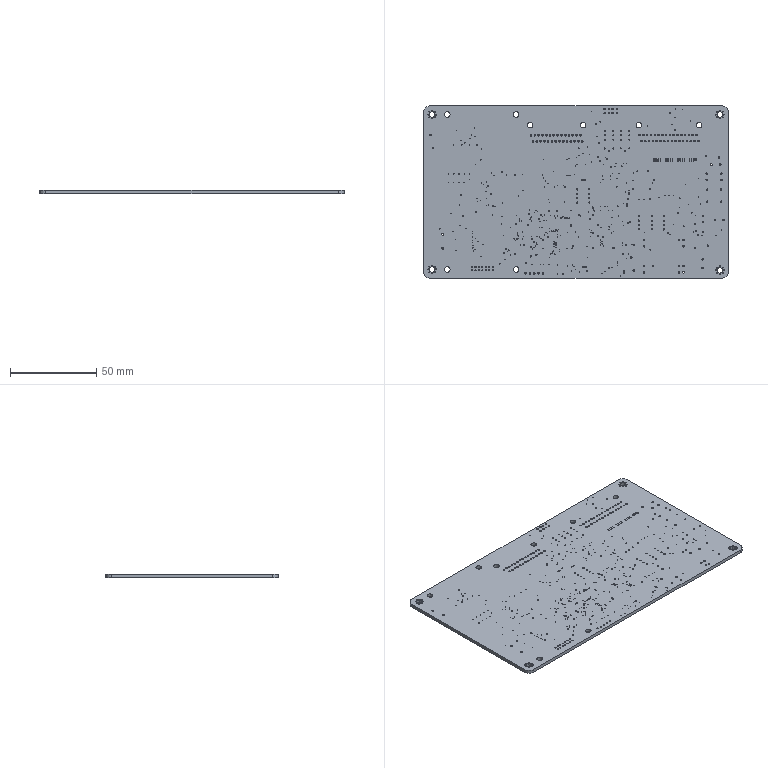Part | SolidWorks | features BaseBody 1 | 1 solid | 1254 faces | box 177 x 100 x 2 mm | volume 34913 mm3 | cylinder 1248 | plane 6 | commonest cylinder face diameters 0.305 x670 0.381 x136 0.889 x104 0.6 x96 0.7 x68 1 x60